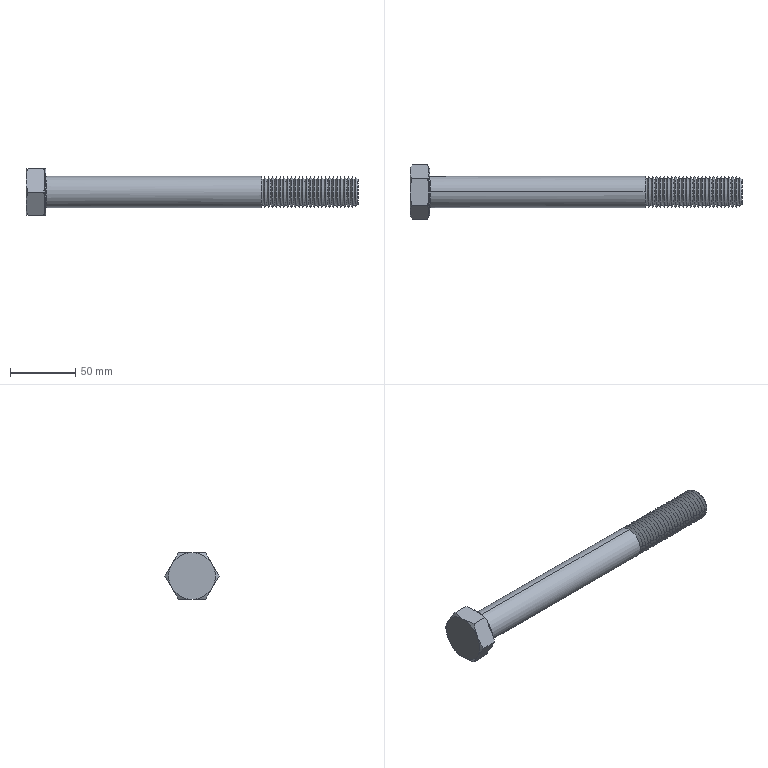Part | SolidWorks | 1 solid | 137 faces | box 255 x 41.569 x 36 mm | volume 118287 mm3 | cone 116 | plane 15 | cylinder 4 | torus 2 | commonest cylinder face diameters 24 x2 36 x2